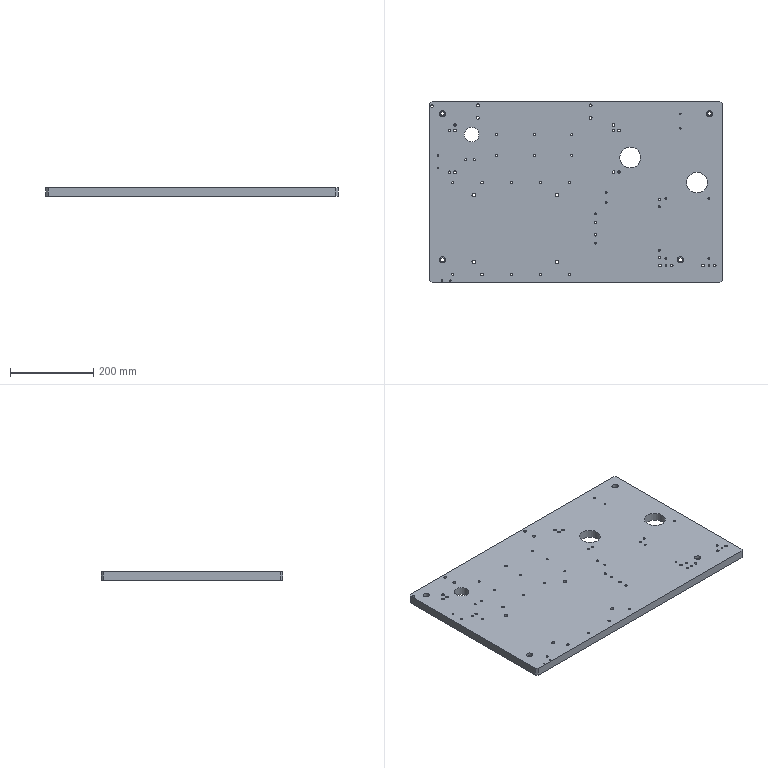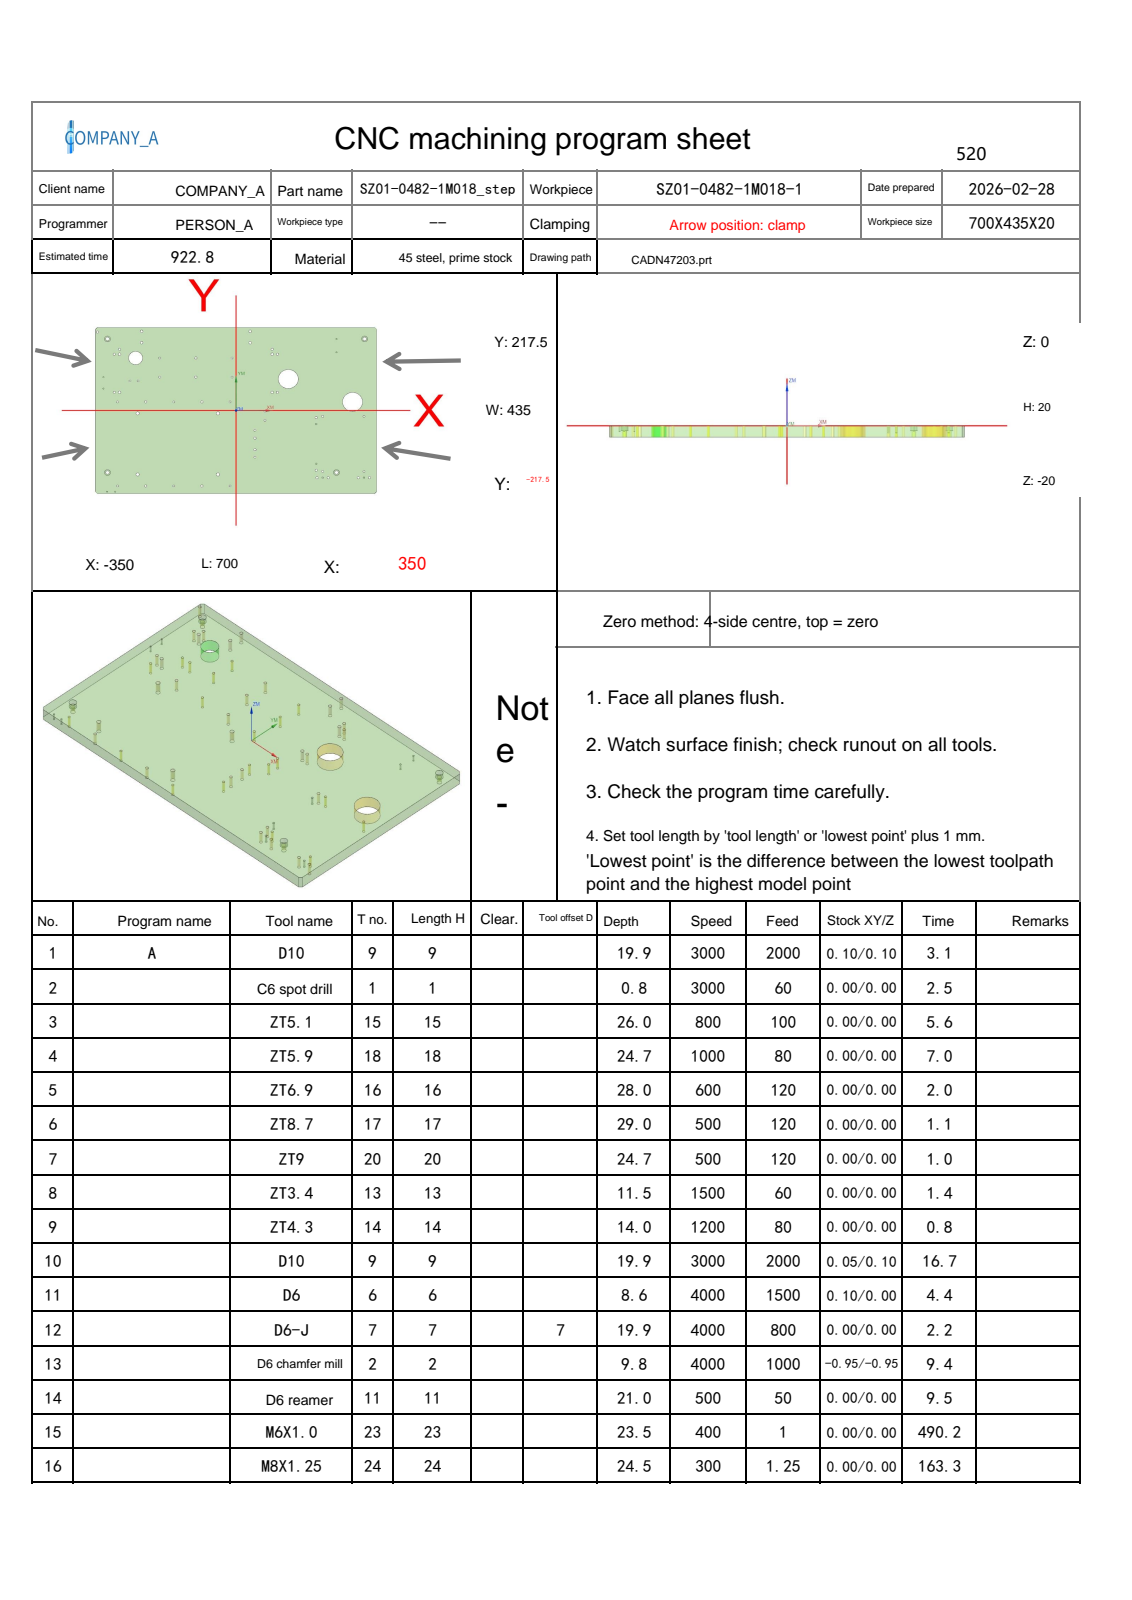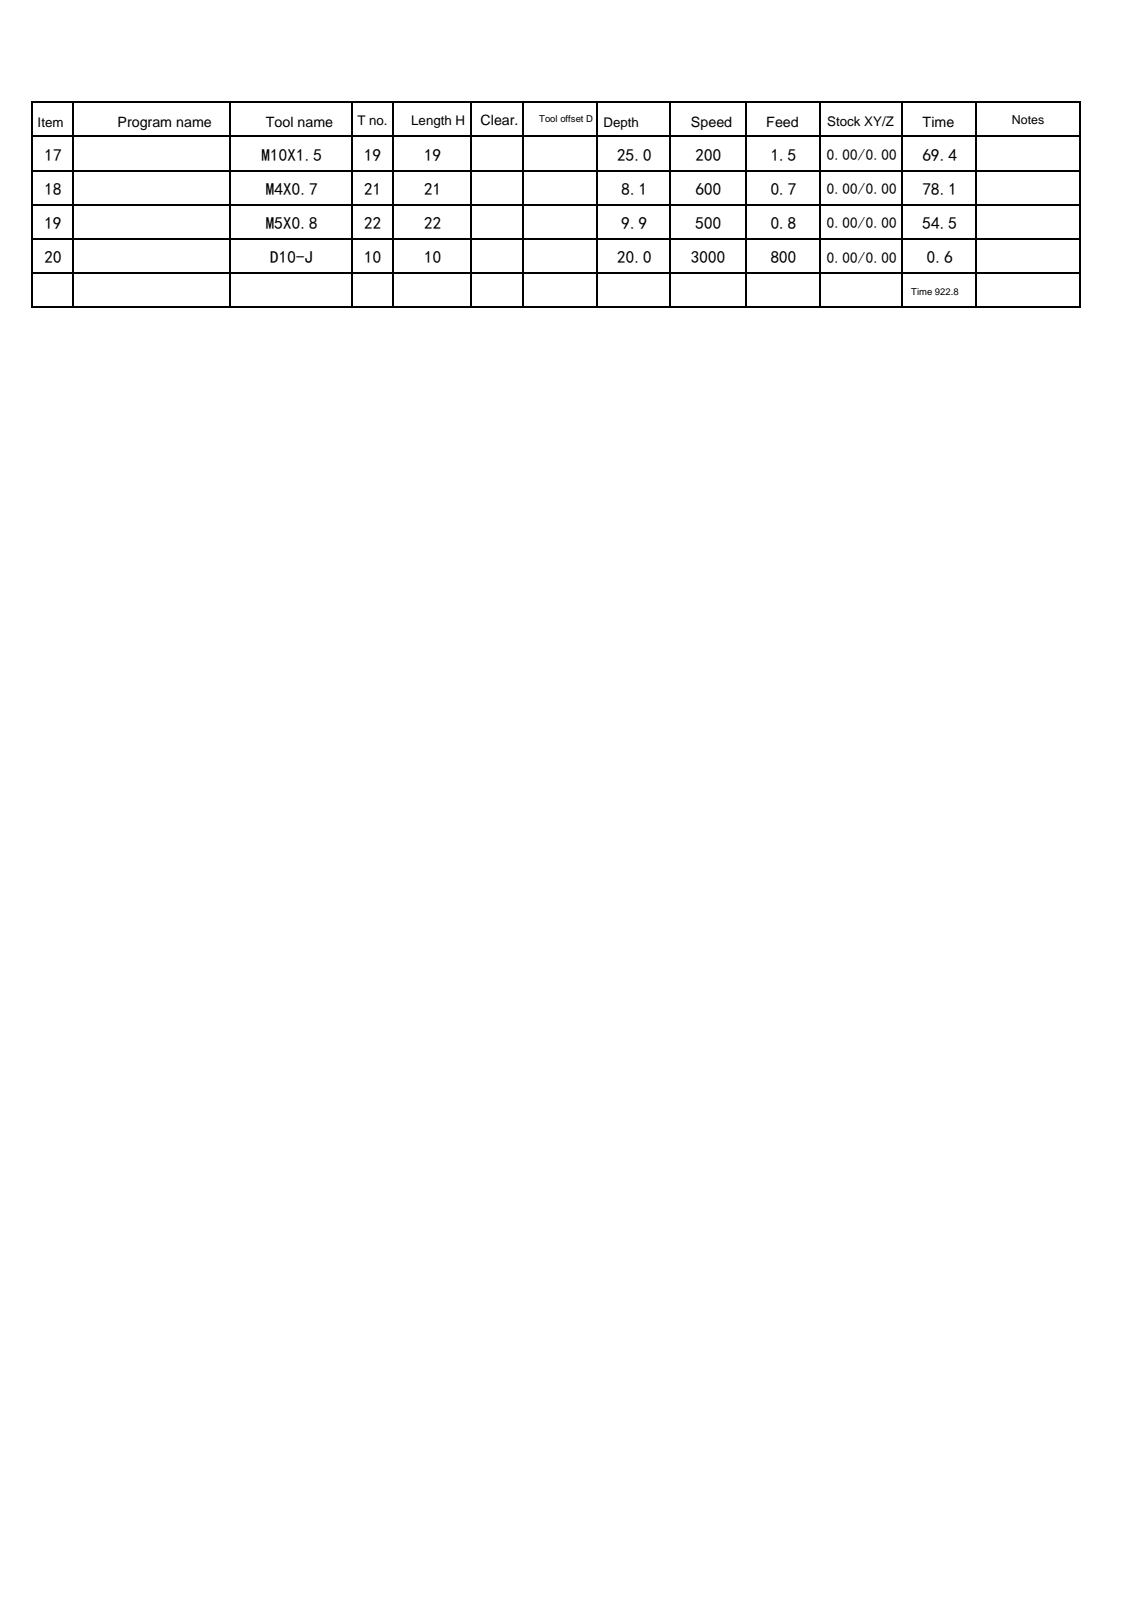NC program | NX | posted by the shop | part box 700 x 435 x 20 mm
Lines 1191 to 2452 of 5271, first 972 of 1262 lines:
N10 T09 M06
(D10  D=10. R=0. H=09 ce=0.05 di=0.10)
G00 G90 G54 X301.511 Y6.205 M03 S3000
G43 H09 Z50.
M08
Z1.
G01 X301.92 Y6.466 Z.975 F2000.
X304.128 Y8.372 Z.822
X306.034 Y10.58 Z.669
X307.599 Y13.041 Z.516
X308.789 Y15.704 Z.363
X309.578 Y18.512 Z.21
X309.95 Y21.406 Z.057
Y22.5 Z0.0
G03 X290. Y42.45 Z-.05 I-19.95 J0.0
X270.05 Y22.5 Z-.099 I0.0 J-19.95
X290. Y2.55 Z-.149 I19.95 J0.0
X309.95 Y22.5 Z-.199 I0.0 J19.95
X290. Y42.45 Z-.248 I-19.95 J0.0
X270.05 Y22.5 Z-.298 I0.0 J-19.95
X290. Y2.55 Z-.347 I19.95 J0.0
X309.95 Y22.5 Z-.397 I0.0 J19.95
X290. Y42.45 Z-.447 I-19.95 J0.0
X270.05 Y22.5 Z-.496 I0.0 J-19.95
X290. Y2.55 Z-.546 I19.95 J0.0
X309.95 Y22.5 Z-.596 I0.0 J19.95
X290. Y42.45 Z-.645 I-19.95 J0.0
X270.05 Y22.5 Z-.695 I0.0 J-19.95
X290. Y2.55 Z-.744 I19.95 J0.0
X309.95 Y22.5 Z-.794 I0.0 J19.95
X290. Y42.45 Z-.844 I-19.95 J0.0
X270.05 Y22.5 Z-.893 I0.0 J-19.95
X290. Y2.55 Z-.943 I19.95 J0.0
X309.95 Y22.5 Z-.993 I0.0 J19.95
X290. Y42.45 Z-1.042 I-19.95 J0.0
X270.05 Y22.5 Z-1.092 I0.0 J-19.95
X290. Y2.55 Z-1.141 I19.95 J0.0
X309.95 Y22.5 Z-1.191 I0.0 J19.95
X290. Y42.45 Z-1.241 I-19.95 J0.0
X270.05 Y22.5 Z-1.29 I0.0 J-19.95
X290. Y2.55 Z-1.34 I19.95 J0.0
X309.95 Y22.5 Z-1.39 I0.0 J19.95
X290. Y42.45 Z-1.439 I-19.95 J0.0
X270.05 Y22.5 Z-1.489 I0.0 J-19.95
X290. Y2.55 Z-1.538 I19.95 J0.0
X309.95 Y22.5 Z-1.588 I0.0 J19.95
X290. Y42.45 Z-1.638 I-19.95 J0.0
X270.05 Y22.5 Z-1.687 I0.0 J-19.95
X290. Y2.55 Z-1.737 I19.95 J0.0
X309.95 Y22.5 Z-1.787 I0.0 J19.95
X290. Y42.45 Z-1.836 I-19.95 J0.0
X270.05 Y22.5 Z-1.886 I0.0 J-19.95
X290. Y2.55 Z-1.935 I19.95 J0.0
X309.95 Y22.5 Z-1.985 I0.0 J19.95
X290. Y42.45 Z-2.035 I-19.95 J0.0
X270.05 Y22.5 Z-2.084 I0.0 J-19.95
X290. Y2.55 Z-2.134 I19.95 J0.0
X309.95 Y22.5 Z-2.184 I0.0 J19.95
X290. Y42.45 Z-2.233 I-19.95 J0.0
X270.05 Y22.5 Z-2.283 I0.0 J-19.95
X290. Y2.55 Z-2.332 I19.95 J0.0
X309.95 Y22.5 Z-2.382 I0.0 J19.95
X290. Y42.45 Z-2.432 I-19.95 J0.0
X270.05 Y22.5 Z-2.481 I0.0 J-19.95
X290. Y2.55 Z-2.531 I19.95 J0.0
X309.95 Y22.5 Z-2.581 I0.0 J19.95
X290. Y42.45 Z-2.63 I-19.95 J0.0
X270.05 Y22.5 Z-2.68 I0.0 J-19.95
X290. Y2.55 Z-2.729 I19.95 J0.0
X309.95 Y22.5 Z-2.779 I0.0 J19.95
X290. Y42.45 Z-2.829 I-19.95 J0.0
X270.05 Y22.5 Z-2.878 I0.0 J-19.95
X290. Y2.55 Z-2.928 I19.95 J0.0
X309.95 Y22.5 Z-2.978 I0.0 J19.95
X290. Y42.45 Z-3.027 I-19.95 J0.0
X270.05 Y22.5 Z-3.077 I0.0 J-19.95
X290. Y2.55 Z-3.126 I19.95 J0.0
X309.95 Y22.5 Z-3.176 I0.0 J19.95
X290. Y42.45 Z-3.226 I-19.95 J0.0
X270.05 Y22.5 Z-3.275 I0.0 J-19.95
X290. Y2.55 Z-3.325 I19.95 J0.0
X309.95 Y22.5 Z-3.375 I0.0 J19.95
X290. Y42.45 Z-3.424 I-19.95 J0.0
X270.05 Y22.5 Z-3.474 I0.0 J-19.95
X290. Y2.55 Z-3.523 I19.95 J0.0
X309.95 Y22.5 Z-3.573 I0.0 J19.95
X290. Y42.45 Z-3.623 I-19.95 J0.0
X270.05 Y22.5 Z-3.672 I0.0 J-19.95
X290. Y2.55 Z-3.722 I19.95 J0.0
X309.95 Y22.5 Z-3.772 I0.0 J19.95
X290. Y42.45 Z-3.821 I-19.95 J0.0
X270.05 Y22.5 Z-3.871 I0.0 J-19.95
X290. Y2.55 Z-3.92 I19.95 J0.0
X309.95 Y22.5 Z-3.97 I0.0 J19.95
X290. Y42.45 Z-4.02 I-19.95 J0.0
X270.05 Y22.5 Z-4.069 I0.0 J-19.95
X290. Y2.55 Z-4.119 I19.95 J0.0
X309.95 Y22.5 Z-4.169 I0.0 J19.95
X290. Y42.45 Z-4.218 I-19.95 J0.0
X270.05 Y22.5 Z-4.268 I0.0 J-19.95
X290. Y2.55 Z-4.317 I19.95 J0.0
X309.95 Y22.5 Z-4.367 I0.0 J19.95
X290. Y42.45 Z-4.417 I-19.95 J0.0
X270.05 Y22.5 Z-4.466 I0.0 J-19.95
X290. Y2.55 Z-4.516 I19.95 J0.0
X309.95 Y22.5 Z-4.566 I0.0 J19.95
X290. Y42.45 Z-4.615 I-19.95 J0.0
X270.05 Y22.5 Z-4.665 I0.0 J-19.95
X290. Y2.55 Z-4.714 I19.95 J0.0
X309.95 Y22.5 Z-4.764 I0.0 J19.95
X290. Y42.45 Z-4.814 I-19.95 J0.0
X270.05 Y22.5 Z-4.863 I0.0 J-19.95
X290. Y2.55 Z-4.913 I19.95 J0.0
X309.95 Y22.5 Z-4.963 I0.0 J19.95
X290. Y42.45 Z-5.012 I-19.95 J0.0
X270.05 Y22.5 Z-5.062 I0.0 J-19.95
X290. Y2.55 Z-5.111 I19.95 J0.0
X309.95 Y22.5 Z-5.161 I0.0 J19.95
X290. Y42.45 Z-5.211 I-19.95 J0.0
X270.05 Y22.5 Z-5.26 I0.0 J-19.95
X290. Y2.55 Z-5.31 I19.95 J0.0
X309.95 Y22.5 Z-5.36 I0.0 J19.95
X290. Y42.45 Z-5.409 I-19.95 J0.0
X270.05 Y22.5 Z-5.459 I0.0 J-19.95
X290. Y2.55 Z-5.508 I19.95 J0.0
X309.95 Y22.5 Z-5.558 I0.0 J19.95
X290. Y42.45 Z-5.608 I-19.95 J0.0
X270.05 Y22.5 Z-5.657 I0.0 J-19.95
X290. Y2.55 Z-5.707 I19.95 J0.0
X309.95 Y22.5 Z-5.757 I0.0 J19.95
X290. Y42.45 Z-5.806 I-19.95 J0.0
X270.05 Y22.5 Z-5.856 I0.0 J-19.95
X290. Y2.55 Z-5.905 I19.95 J0.0
X309.95 Y22.5 Z-5.955 I0.0 J19.95
X290. Y42.45 Z-6.005 I-19.95 J0.0
X270.05 Y22.5 Z-6.054 I0.0 J-19.95
X290. Y2.55 Z-6.104 I19.95 J0.0
X309.95 Y22.5 Z-6.154 I0.0 J19.95
X290. Y42.45 Z-6.203 I-19.95 J0.0
X270.05 Y22.5 Z-6.253 I0.0 J-19.95
X290. Y2.55 Z-6.302 I19.95 J0.0
X309.95 Y22.5 Z-6.352 I0.0 J19.95
X290. Y42.45 Z-6.402 I-19.95 J0.0
X270.05 Y22.5 Z-6.451 I0.0 J-19.95
X290. Y2.55 Z-6.501 I19.95 J0.0
X309.95 Y22.5 Z-6.551 I0.0 J19.95
X290. Y42.45 Z-6.6 I-19.95 J0.0
X270.05 Y22.5 Z-6.65 I0.0 J-19.95
X290. Y2.55 Z-6.699 I19.95 J0.0
X309.95 Y22.5 Z-6.749 I0.0 J19.95
X290. Y42.45 Z-6.799 I-19.95 J0.0
X270.05 Y22.5 Z-6.848 I0.0 J-19.95
X290. Y2.55 Z-6.898 I19.95 J0.0
X309.95 Y22.5 Z-6.948 I0.0 J19.95
X290. Y42.45 Z-6.997 I-19.95 J0.0
X270.05 Y22.5 Z-7.047 I0.0 J-19.95
X290. Y2.55 Z-7.096 I19.95 J0.0
X309.95 Y22.5 Z-7.146 I0.0 J19.95
X290. Y42.45 Z-7.196 I-19.95 J0.0
X270.05 Y22.5 Z-7.245 I0.0 J-19.95
X290. Y2.55 Z-7.295 I19.95 J0.0
X309.95 Y22.5 Z-7.345 I0.0 J19.95
X290. Y42.45 Z-7.394 I-19.95 J0.0
X270.05 Y22.5 Z-7.444 I0.0 J-19.95
X290. Y2.55 Z-7.493 I19.95 J0.0
X309.95 Y22.5 Z-7.543 I0.0 J19.95
X290. Y42.45 Z-7.593 I-19.95 J0.0
X270.05 Y22.5 Z-7.642 I0.0 J-19.95
X290. Y2.55 Z-7.692 I19.95 J0.0
X309.95 Y22.5 Z-7.742 I0.0 J19.95
X290. Y42.45 Z-7.791 I-19.95 J0.0
X270.05 Y22.5 Z-7.841 I0.0 J-19.95
X290. Y2.55 Z-7.89 I19.95 J0.0
X309.95 Y22.5 Z-7.94 I0.0 J19.95
X290. Y42.45 Z-7.99 I-19.95 J0.0
X270.05 Y22.5 Z-8.039 I0.0 J-19.95
X290. Y2.55 Z-8.089 I19.95 J0.0
X309.95 Y22.5 Z-8.139 I0.0 J19.95
X290. Y42.45 Z-8.188 I-19.95 J0.0
X270.05 Y22.5 Z-8.238 I0.0 J-19.95
X290. Y2.55 Z-8.287 I19.95 J0.0
X309.95 Y22.5 Z-8.337 I0.0 J19.95
X290. Y42.45 Z-8.387 I-19.95 J0.0
X270.05 Y22.5 Z-8.436 I0.0 J-19.95
X290. Y2.55 Z-8.486 I19.95 J0.0
X309.95 Y22.5 Z-8.536 I0.0 J19.95
X290. Y42.45 Z-8.585 I-19.95 J0.0
X270.05 Y22.5 Z-8.635 I0.0 J-19.95
X290. Y2.55 Z-8.684 I19.95 J0.0
X309.95 Y22.5 Z-8.734 I0.0 J19.95
X290. Y42.45 Z-8.784 I-19.95 J0.0
X270.05 Y22.5 Z-8.833 I0.0 J-19.95
X290. Y2.55 Z-8.883 I19.95 J0.0
X309.95 Y22.5 Z-8.933 I0.0 J19.95
X290. Y42.45 Z-8.982 I-19.95 J0.0
X270.05 Y22.5 Z-9.032 I0.0 J-19.95
X290. Y2.55 Z-9.081 I19.95 J0.0
X309.95 Y22.5 Z-9.131 I0.0 J19.95
X290. Y42.45 Z-9.181 I-19.95 J0.0
X270.05 Y22.5 Z-9.23 I0.0 J-19.95
X290. Y2.55 Z-9.28 I19.95 J0.0
X309.95 Y22.5 Z-9.33 I0.0 J19.95
X290. Y42.45 Z-9.379 I-19.95 J0.0
X270.05 Y22.5 Z-9.429 I0.0 J-19.95
X290. Y2.55 Z-9.478 I19.95 J0.0
X309.95 Y22.5 Z-9.528 I0.0 J19.95
X290. Y42.45 Z-9.578 I-19.95 J0.0
X270.05 Y22.5 Z-9.627 I0.0 J-19.95
X290. Y2.55 Z-9.677 I19.95 J0.0
X309.95 Y22.5 Z-9.727 I0.0 J19.95
X290. Y42.45 Z-9.776 I-19.95 J0.0
X270.05 Y22.5 Z-9.826 I0.0 J-19.95
X290. Y2.55 Z-9.875 I19.95 J0.0
X309.95 Y22.5 Z-9.925 I0.0 J19.95
X290. Y42.45 Z-9.975 I-19.95 J0.0
X270.05 Y22.5 Z-10.024 I0.0 J-19.95
X290. Y2.55 Z-10.074 I19.95 J0.0
X309.95 Y22.5 Z-10.124 I0.0 J19.95
X290. Y42.45 Z-10.173 I-19.95 J0.0
X270.05 Y22.5 Z-10.223 I0.0 J-19.95
X290. Y2.55 Z-10.272 I19.95 J0.0
X309.95 Y22.5 Z-10.322 I0.0 J19.95
X290. Y42.45 Z-10.372 I-19.95 J0.0
X270.05 Y22.5 Z-10.421 I0.0 J-19.95
X290. Y2.55 Z-10.471 I19.95 J0.0
X309.95 Y22.5 Z-10.521 I0.0 J19.95
X290. Y42.45 Z-10.57 I-19.95 J0.0
X270.05 Y22.5 Z-10.62 I0.0 J-19.95
X290. Y2.55 Z-10.669 I19.95 J0.0
X309.95 Y22.5 Z-10.719 I0.0 J19.95
X290. Y42.45 Z-10.769 I-19.95 J0.0
X270.05 Y22.5 Z-10.818 I0.0 J-19.95
X290. Y2.55 Z-10.868 I19.95 J0.0
X309.95 Y22.5 Z-10.918 I0.0 J19.95
X290. Y42.45 Z-10.967 I-19.95 J0.0
X270.05 Y22.5 Z-11.017 I0.0 J-19.95
X290. Y2.55 Z-11.066 I19.95 J0.0
X309.95 Y22.5 Z-11.116 I0.0 J19.95
X290. Y42.45 Z-11.166 I-19.95 J0.0
X270.05 Y22.5 Z-11.215 I0.0 J-19.95
X290. Y2.55 Z-11.265 I19.95 J0.0
X309.95 Y22.5 Z-11.315 I0.0 J19.95
X290. Y42.45 Z-11.364 I-19.95 J0.0
X270.05 Y22.5 Z-11.414 I0.0 J-19.95
X290. Y2.55 Z-11.463 I19.95 J0.0
X309.95 Y22.5 Z-11.513 I0.0 J19.95
X290. Y42.45 Z-11.563 I-19.95 J0.0
X270.05 Y22.5 Z-11.612 I0.0 J-19.95
X290. Y2.55 Z-11.662 I19.95 J0.0
X309.95 Y22.5 Z-11.712 I0.0 J19.95
X290. Y42.45 Z-11.761 I-19.95 J0.0
X270.05 Y22.5 Z-11.811 I0.0 J-19.95
X290. Y2.55 Z-11.86 I19.95 J0.0
X309.95 Y22.5 Z-11.91 I0.0 J19.95
X290. Y42.45 Z-11.96 I-19.95 J0.0
X270.05 Y22.5 Z-12.009 I0.0 J-19.95
X290. Y2.55 Z-12.059 I19.95 J0.0
X309.95 Y22.5 Z-12.109 I0.0 J19.95
X290. Y42.45 Z-12.158 I-19.95 J0.0
X270.05 Y22.5 Z-12.208 I0.0 J-19.95
X290. Y2.55 Z-12.257 I19.95 J0.0
X309.95 Y22.5 Z-12.307 I0.0 J19.95
X290. Y42.45 Z-12.357 I-19.95 J0.0
X270.05 Y22.5 Z-12.406 I0.0 J-19.95
X290. Y2.55 Z-12.456 I19.95 J0.0
X309.95 Y22.5 Z-12.506 I0.0 J19.95
X290. Y42.45 Z-12.555 I-19.95 J0.0
X270.05 Y22.5 Z-12.605 I0.0 J-19.95
X290. Y2.55 Z-12.654 I19.95 J0.0
X309.95 Y22.5 Z-12.704 I0.0 J19.95
X290. Y42.45 Z-12.754 I-19.95 J0.0
X270.05 Y22.5 Z-12.803 I0.0 J-19.95
X290. Y2.55 Z-12.853 I19.95 J0.0
X309.95 Y22.5 Z-12.903 I0.0 J19.95
X290. Y42.45 Z-12.952 I-19.95 J0.0
X270.05 Y22.5 Z-13.002 I0.0 J-19.95
X290. Y2.55 Z-13.051 I19.95 J0.0
X309.95 Y22.5 Z-13.101 I0.0 J19.95
X290. Y42.45 Z-13.151 I-19.95 J0.0
X270.05 Y22.5 Z-13.2 I0.0 J-19.95
X290. Y2.55 Z-13.25 I19.95 J0.0
X309.95 Y22.5 Z-13.3 I0.0 J19.95
X290. Y42.45 Z-13.349 I-19.95 J0.0
X270.05 Y22.5 Z-13.399 I0.0 J-19.95
X290. Y2.55 Z-13.448 I19.95 J0.0
X309.95 Y22.5 Z-13.498 I0.0 J19.95
X290. Y42.45 Z-13.548 I-19.95 J0.0
X270.05 Y22.5 Z-13.597 I0.0 J-19.95
X290. Y2.55 Z-13.647 I19.95 J0.0
X309.95 Y22.5 Z-13.697 I0.0 J19.95
X290. Y42.45 Z-13.746 I-19.95 J0.0
X270.05 Y22.5 Z-13.796 I0.0 J-19.95
X290. Y2.55 Z-13.845 I19.95 J0.0
X309.95 Y22.5 Z-13.895 I0.0 J19.95
X290. Y42.45 Z-13.945 I-19.95 J0.0
X270.05 Y22.5 Z-13.994 I0.0 J-19.95
X290. Y2.55 Z-14.044 I19.95 J0.0
X309.95 Y22.5 Z-14.094 I0.0 J19.95
X290. Y42.45 Z-14.143 I-19.95 J0.0
X270.05 Y22.5 Z-14.193 I0.0 J-19.95
X290. Y2.55 Z-14.242 I19.95 J0.0
X309.95 Y22.5 Z-14.292 I0.0 J19.95
X290. Y42.45 Z-14.342 I-19.95 J0.0
X270.05 Y22.5 Z-14.391 I0.0 J-19.95
X290. Y2.55 Z-14.441 I19.95 J0.0
X309.95 Y22.5 Z-14.491 I0.0 J19.95
X290. Y42.45 Z-14.54 I-19.95 J0.0
X270.05 Y22.5 Z-14.59 I0.0 J-19.95
X290. Y2.55 Z-14.639 I19.95 J0.0
X309.95 Y22.5 Z-14.689 I0.0 J19.95
X290. Y42.45 Z-14.739 I-19.95 J0.0
X270.05 Y22.5 Z-14.788 I0.0 J-19.95
X290. Y2.55 Z-14.838 I19.95 J0.0
X309.95 Y22.5 Z-14.888 I0.0 J19.95
X290. Y42.45 Z-14.937 I-19.95 J0.0
X270.05 Y22.5 Z-14.987 I0.0 J-19.95
X290. Y2.55 Z-15.036 I19.95 J0.0
X309.95 Y22.5 Z-15.086 I0.0 J19.95
X290. Y42.45 Z-15.136 I-19.95 J0.0
X270.05 Y22.5 Z-15.185 I0.0 J-19.95
X290. Y2.55 Z-15.235 I19.95 J0.0
X309.95 Y22.5 Z-15.285 I0.0 J19.95
X290. Y42.45 Z-15.334 I-19.95 J0.0
X270.05 Y22.5 Z-15.384 I0.0 J-19.95
X290. Y2.55 Z-15.433 I19.95 J0.0
X309.95 Y22.5 Z-15.483 I0.0 J19.95
X290. Y42.45 Z-15.533 I-19.95 J0.0
X270.05 Y22.5 Z-15.582 I0.0 J-19.95
X290. Y2.55 Z-15.632 I19.95 J0.0
X309.95 Y22.5 Z-15.682 I0.0 J19.95
X290. Y42.45 Z-15.731 I-19.95 J0.0
X270.05 Y22.5 Z-15.781 I0.0 J-19.95
X290. Y2.55 Z-15.83 I19.95 J0.0
X309.95 Y22.5 Z-15.88 I0.0 J19.95
X290. Y42.45 Z-15.93 I-19.95 J0.0
X270.05 Y22.5 Z-15.979 I0.0 J-19.95
X290. Y2.55 Z-16.029 I19.95 J0.0
X309.95 Y22.5 Z-16.079 I0.0 J19.95
X290. Y42.45 Z-16.128 I-19.95 J0.0
X270.05 Y22.5 Z-16.178 I0.0 J-19.95
X290. Y2.55 Z-16.227 I19.95 J0.0
X309.95 Y22.5 Z-16.277 I0.0 J19.95
X290. Y42.45 Z-16.327 I-19.95 J0.0
X270.05 Y22.5 Z-16.376 I0.0 J-19.95
X290. Y2.55 Z-16.426 I19.95 J0.0
X309.95 Y22.5 Z-16.476 I0.0 J19.95
X290. Y42.45 Z-16.525 I-19.95 J0.0
X270.05 Y22.5 Z-16.575 I0.0 J-19.95
X290. Y2.55 Z-16.624 I19.95 J0.0
X309.95 Y22.5 Z-16.674 I0.0 J19.95
X290. Y42.45 Z-16.724 I-19.95 J0.0
X270.05 Y22.5 Z-16.773 I0.0 J-19.95
X290. Y2.55 Z-16.823 I19.95 J0.0
X309.95 Y22.5 Z-16.873 I0.0 J19.95
X290. Y42.45 Z-16.922 I-19.95 J0.0
X270.05 Y22.5 Z-16.972 I0.0 J-19.95
X290. Y2.55 Z-17.021 I19.95 J0.0
X309.95 Y22.5 Z-17.071 I0.0 J19.95
X290. Y42.45 Z-17.121 I-19.95 J0.0
X270.05 Y22.5 Z-17.17 I0.0 J-19.95
X290. Y2.55 Z-17.22 I19.95 J0.0
X309.95 Y22.5 Z-17.27 I0.0 J19.95
X290. Y42.45 Z-17.319 I-19.95 J0.0
X270.05 Y22.5 Z-17.369 I0.0 J-19.95
X290. Y2.55 Z-17.418 I19.95 J0.0
X309.95 Y22.5 Z-17.468 I0.0 J19.95
X290. Y42.45 Z-17.518 I-19.95 J0.0
X270.05 Y22.5 Z-17.567 I0.0 J-19.95
X290. Y2.55 Z-17.617 I19.95 J0.0
X309.95 Y22.5 Z-17.667 I0.0 J19.95
X290. Y42.45 Z-17.716 I-19.95 J0.0
X270.05 Y22.5 Z-17.766 I0.0 J-19.95
X290. Y2.55 Z-17.815 I19.95 J0.0
X309.95 Y22.5 Z-17.865 I0.0 J19.95
X290. Y42.45 Z-17.915 I-19.95 J0.0
X270.05 Y22.5 Z-17.964 I0.0 J-19.95
X290. Y2.55 Z-18.014 I19.95 J0.0
X309.95 Y22.5 Z-18.064 I0.0 J19.95
X290. Y42.45 Z-18.113 I-19.95 J0.0
X270.05 Y22.5 Z-18.163 I0.0 J-19.95
X290. Y2.55 Z-18.212 I19.95 J0.0
X309.95 Y22.5 Z-18.262 I0.0 J19.95
X290. Y42.45 Z-18.312 I-19.95 J0.0
X270.05 Y22.5 Z-18.361 I0.0 J-19.95
X290. Y2.55 Z-18.411 I19.95 J0.0
X309.95 Y22.5 Z-18.461 I0.0 J19.95
X290. Y42.45 Z-18.51 I-19.95 J0.0
X270.05 Y22.5 Z-18.56 I0.0 J-19.95
X290. Y2.55 Z-18.609 I19.95 J0.0
X309.95 Y22.5 Z-18.659 I0.0 J19.95
X290. Y42.45 Z-18.709 I-19.95 J0.0
X270.05 Y22.5 Z-18.758 I0.0 J-19.95
X290. Y2.55 Z-18.808 I19.95 J0.0
X309.95 Y22.5 Z-18.858 I0.0 J19.95
X290. Y42.45 Z-18.907 I-19.95 J0.0
X270.05 Y22.5 Z-18.957 I0.0 J-19.95
X290. Y2.55 Z-19.006 I19.95 J0.0
X309.95 Y22.5 Z-19.056 I0.0 J19.95
X290. Y42.45 Z-19.106 I-19.95 J0.0
X270.05 Y22.5 Z-19.155 I0.0 J-19.95
X290. Y2.55 Z-19.205 I19.95 J0.0
X309.95 Y22.5 Z-19.255 I0.0 J19.95
X290. Y42.45 Z-19.304 I-19.95 J0.0
X270.05 Y22.5 Z-19.354 I0.0 J-19.95
X290. Y2.55 Z-19.403 I19.95 J0.0
X309.95 Y22.5 Z-19.453 I0.0 J19.95
X290. Y42.45 Z-19.503 I-19.95 J0.0
X270.05 Y22.5 Z-19.552 I0.0 J-19.95
X290. Y2.55 Z-19.602 I19.95 J0.0
X309.95 Y22.5 Z-19.652 I0.0 J19.95
X290. Y42.45 Z-19.701 I-19.95 J0.0
X270.05 Y22.5 Z-19.751 I0.0 J-19.95
X290. Y2.55 Z-19.8 I19.95 J0.0
X309.95 Y22.5 Z-19.85 I0.0 J19.95
X290. Y42.45 I-19.95 J0.0
X270.05 Y22.5 I0.0 J-19.95
X290. Y2.55 I19.95 J0.0
X309.95 Y22.5 I0.0 J19.95
X309.946 Y22.9 I-19.95 J0.0
G01 Z-18.85
G00 Z50.
X146.295 Y94.011
Z1.
G01 X146.034 Y94.42 Z.975
X144.128 Y96.628 Z.822
X141.92 Y98.534 Z.669
X139.459 Y100.099 Z.516
X136.796 Y101.289 Z.363
X133.988 Y102.078 Z.21
X131.094 Y102.45 Z.057
X130. Z0.0
G03 X110.05 Y82.5 Z-.05 I0.0 J-19.95
X130. Y62.55 Z-.099 I19.95 J0.0
X149.95 Y82.5 Z-.149 I0.0 J19.95
X130. Y102.45 Z-.199 I-19.95 J0.0
X110.05 Y82.5 Z-.248 I0.0 J-19.95
X130. Y62.55 Z-.298 I19.95 J0.0
X149.95 Y82.5 Z-.347 I0.0 J19.95
X130. Y102.45 Z-.397 I-19.95 J0.0
X110.05 Y82.5 Z-.447 I0.0 J-19.95
X130. Y62.55 Z-.496 I19.95 J0.0
X149.95 Y82.5 Z-.546 I0.0 J19.95
X130. Y102.45 Z-.596 I-19.95 J0.0
X110.05 Y82.5 Z-.645 I0.0 J-19.95
X130. Y62.55 Z-.695 I19.95 J0.0
X149.95 Y82.5 Z-.744 I0.0 J19.95
X130. Y102.45 Z-.794 I-19.95 J0.0
X110.05 Y82.5 Z-.844 I0.0 J-19.95
X130. Y62.55 Z-.893 I19.95 J0.0
X149.95 Y82.5 Z-.943 I0.0 J19.95
X130. Y102.45 Z-.993 I-19.95 J0.0
X110.05 Y82.5 Z-1.042 I0.0 J-19.95
X130. Y62.55 Z-1.092 I19.95 J0.0
X149.95 Y82.5 Z-1.141 I0.0 J19.95
X130. Y102.45 Z-1.191 I-19.95 J0.0
X110.05 Y82.5 Z-1.241 I0.0 J-19.95
X130. Y62.55 Z-1.29 I19.95 J0.0
X149.95 Y82.5 Z-1.34 I0.0 J19.95
X130. Y102.45 Z-1.39 I-19.95 J0.0
X110.05 Y82.5 Z-1.439 I0.0 J-19.95
X130. Y62.55 Z-1.489 I19.95 J0.0
X149.95 Y82.5 Z-1.538 I0.0 J19.95
X130. Y102.45 Z-1.588 I-19.95 J0.0
X110.05 Y82.5 Z-1.638 I0.0 J-19.95
X130. Y62.55 Z-1.687 I19.95 J0.0
X149.95 Y82.5 Z-1.737 I0.0 J19.95
X130. Y102.45 Z-1.787 I-19.95 J0.0
X110.05 Y82.5 Z-1.836 I0.0 J-19.95
X130. Y62.55 Z-1.886 I19.95 J0.0
X149.95 Y82.5 Z-1.935 I0.0 J19.95
X130. Y102.45 Z-1.985 I-19.95 J0.0
X110.05 Y82.5 Z-2.035 I0.0 J-19.95
X130. Y62.55 Z-2.084 I19.95 J0.0
X149.95 Y82.5 Z-2.134 I0.0 J19.95
X130. Y102.45 Z-2.184 I-19.95 J0.0
X110.05 Y82.5 Z-2.233 I0.0 J-19.95
X130. Y62.55 Z-2.283 I19.95 J0.0
X149.95 Y82.5 Z-2.332 I0.0 J19.95
X130. Y102.45 Z-2.382 I-19.95 J0.0
X110.05 Y82.5 Z-2.432 I0.0 J-19.95
X130. Y62.55 Z-2.481 I19.95 J0.0
X149.95 Y82.5 Z-2.531 I0.0 J19.95
X130. Y102.45 Z-2.581 I-19.95 J0.0
X110.05 Y82.5 Z-2.63 I0.0 J-19.95
X130. Y62.55 Z-2.68 I19.95 J0.0
X149.95 Y82.5 Z-2.729 I0.0 J19.95
X130. Y102.45 Z-2.779 I-19.95 J0.0
X110.05 Y82.5 Z-2.829 I0.0 J-19.95
X130. Y62.55 Z-2.878 I19.95 J0.0
X149.95 Y82.5 Z-2.928 I0.0 J19.95
X130. Y102.45 Z-2.978 I-19.95 J0.0
X110.05 Y82.5 Z-3.027 I0.0 J-19.95
X130. Y62.55 Z-3.077 I19.95 J0.0
X149.95 Y82.5 Z-3.126 I0.0 J19.95
X130. Y102.45 Z-3.176 I-19.95 J0.0
X110.05 Y82.5 Z-3.226 I0.0 J-19.95
X130. Y62.55 Z-3.275 I19.95 J0.0
X149.95 Y82.5 Z-3.325 I0.0 J19.95
X130. Y102.45 Z-3.375 I-19.95 J0.0
X110.05 Y82.5 Z-3.424 I0.0 J-19.95
X130. Y62.55 Z-3.474 I19.95 J0.0
X149.95 Y82.5 Z-3.523 I0.0 J19.95
X130. Y102.45 Z-3.573 I-19.95 J0.0
X110.05 Y82.5 Z-3.623 I0.0 J-19.95
X130. Y62.55 Z-3.672 I19.95 J0.0
X149.95 Y82.5 Z-3.722 I0.0 J19.95
X130. Y102.45 Z-3.772 I-19.95 J0.0
X110.05 Y82.5 Z-3.821 I0.0 J-19.95
X130. Y62.55 Z-3.871 I19.95 J0.0
X149.95 Y82.5 Z-3.92 I0.0 J19.95
X130. Y102.45 Z-3.97 I-19.95 J0.0
X110.05 Y82.5 Z-4.02 I0.0 J-19.95
X130. Y62.55 Z-4.069 I19.95 J0.0
X149.95 Y82.5 Z-4.119 I0.0 J19.95
X130. Y102.45 Z-4.169 I-19.95 J0.0
X110.05 Y82.5 Z-4.218 I0.0 J-19.95
X130. Y62.55 Z-4.268 I19.95 J0.0
X149.95 Y82.5 Z-4.317 I0.0 J19.95
X130. Y102.45 Z-4.367 I-19.95 J0.0
X110.05 Y82.5 Z-4.417 I0.0 J-19.95
X130. Y62.55 Z-4.466 I19.95 J0.0
X149.95 Y82.5 Z-4.516 I0.0 J19.95
X130. Y102.45 Z-4.566 I-19.95 J0.0
X110.05 Y82.5 Z-4.615 I0.0 J-19.95
X130. Y62.55 Z-4.665 I19.95 J0.0
X149.95 Y82.5 Z-4.714 I0.0 J19.95
X130. Y102.45 Z-4.764 I-19.95 J0.0
X110.05 Y82.5 Z-4.814 I0.0 J-19.95
X130. Y62.55 Z-4.863 I19.95 J0.0
X149.95 Y82.5 Z-4.913 I0.0 J19.95
X130. Y102.45 Z-4.963 I-19.95 J0.0
X110.05 Y82.5 Z-5.012 I0.0 J-19.95
X130. Y62.55 Z-5.062 I19.95 J0.0
X149.95 Y82.5 Z-5.111 I0.0 J19.95
X130. Y102.45 Z-5.161 I-19.95 J0.0
X110.05 Y82.5 Z-5.211 I0.0 J-19.95
X130. Y62.55 Z-5.26 I19.95 J0.0
X149.95 Y82.5 Z-5.31 I0.0 J19.95
X130. Y102.45 Z-5.36 I-19.95 J0.0
X110.05 Y82.5 Z-5.409 I0.0 J-19.95
X130. Y62.55 Z-5.459 I19.95 J0.0
X149.95 Y82.5 Z-5.508 I0.0 J19.95
X130. Y102.45 Z-5.558 I-19.95 J0.0
X110.05 Y82.5 Z-5.608 I0.0 J-19.95
X130. Y62.55 Z-5.657 I19.95 J0.0
X149.95 Y82.5 Z-5.707 I0.0 J19.95
X130. Y102.45 Z-5.757 I-19.95 J0.0
X110.05 Y82.5 Z-5.806 I0.0 J-19.95
X130. Y62.55 Z-5.856 I19.95 J0.0
X149.95 Y82.5 Z-5.905 I0.0 J19.95
X130. Y102.45 Z-5.955 I-19.95 J0.0
X110.05 Y82.5 Z-6.005 I0.0 J-19.95
X130. Y62.55 Z-6.054 I19.95 J0.0
X149.95 Y82.5 Z-6.104 I0.0 J19.95
X130. Y102.45 Z-6.154 I-19.95 J0.0
X110.05 Y82.5 Z-6.203 I0.0 J-19.95
X130. Y62.55 Z-6.253 I19.95 J0.0
X149.95 Y82.5 Z-6.302 I0.0 J19.95
X130. Y102.45 Z-6.352 I-19.95 J0.0
X110.05 Y82.5 Z-6.402 I0.0 J-19.95
X130. Y62.55 Z-6.451 I19.95 J0.0
X149.95 Y82.5 Z-6.501 I0.0 J19.95
X130. Y102.45 Z-6.551 I-19.95 J0.0
X110.05 Y82.5 Z-6.6 I0.0 J-19.95
X130. Y62.55 Z-6.65 I19.95 J0.0
X149.95 Y82.5 Z-6.699 I0.0 J19.95
X130. Y102.45 Z-6.749 I-19.95 J0.0
X110.05 Y82.5 Z-6.799 I0.0 J-19.95
X130. Y62.55 Z-6.848 I19.95 J0.0
X149.95 Y82.5 Z-6.898 I0.0 J19.95
X130. Y102.45 Z-6.948 I-19.95 J0.0
X110.05 Y82.5 Z-6.997 I0.0 J-19.95
X130. Y62.55 Z-7.047 I19.95 J0.0
X149.95 Y82.5 Z-7.096 I0.0 J19.95
X130. Y102.45 Z-7.146 I-19.95 J0.0
X110.05 Y82.5 Z-7.196 I0.0 J-19.95
X130. Y62.55 Z-7.245 I19.95 J0.0
X149.95 Y82.5 Z-7.295 I0.0 J19.95
X130. Y102.45 Z-7.345 I-19.95 J0.0
X110.05 Y82.5 Z-7.394 I0.0 J-19.95
X130. Y62.55 Z-7.444 I19.95 J0.0
X149.95 Y82.5 Z-7.493 I0.0 J19.95
X130. Y102.45 Z-7.543 I-19.95 J0.0
X110.05 Y82.5 Z-7.593 I0.0 J-19.95
X130. Y62.55 Z-7.642 I19.95 J0.0
X149.95 Y82.5 Z-7.692 I0.0 J19.95
X130. Y102.45 Z-7.742 I-19.95 J0.0
X110.05 Y82.5 Z-7.791 I0.0 J-19.95
X130. Y62.55 Z-7.841 I19.95 J0.0
X149.95 Y82.5 Z-7.89 I0.0 J19.95
X130. Y102.45 Z-7.94 I-19.95 J0.0
X110.05 Y82.5 Z-7.99 I0.0 J-19.95
X130. Y62.55 Z-8.039 I19.95 J0.0
X149.95 Y82.5 Z-8.089 I0.0 J19.95
X130. Y102.45 Z-8.139 I-19.95 J0.0
X110.05 Y82.5 Z-8.188 I0.0 J-19.95
X130. Y62.55 Z-8.238 I19.95 J0.0
X149.95 Y82.5 Z-8.287 I0.0 J19.95
X130. Y102.45 Z-8.337 I-19.95 J0.0
X110.05 Y82.5 Z-8.387 I0.0 J-19.95
X130. Y62.55 Z-8.436 I19.95 J0.0
X149.95 Y82.5 Z-8.486 I0.0 J19.95
X130. Y102.45 Z-8.536 I-19.95 J0.0
X110.05 Y82.5 Z-8.585 I0.0 J-19.95
X130. Y62.55 Z-8.635 I19.95 J0.0
X149.95 Y82.5 Z-8.684 I0.0 J19.95
X130. Y102.45 Z-8.734 I-19.95 J0.0
X110.05 Y82.5 Z-8.784 I0.0 J-19.95
X130. Y62.55 Z-8.833 I19.95 J0.0
X149.95 Y82.5 Z-8.883 I0.0 J19.95
X130. Y102.45 Z-8.933 I-19.95 J0.0
X110.05 Y82.5 Z-8.982 I0.0 J-19.95
X130. Y62.55 Z-9.032 I19.95 J0.0
X149.95 Y82.5 Z-9.081 I0.0 J19.95
X130. Y102.45 Z-9.131 I-19.95 J0.0
X110.05 Y82.5 Z-9.181 I0.0 J-19.95
X130. Y62.55 Z-9.23 I19.95 J0.0
X149.95 Y82.5 Z-9.28 I0.0 J19.95
X130. Y102.45 Z-9.33 I-19.95 J0.0
X110.05 Y82.5 Z-9.379 I0.0 J-19.95
X130. Y62.55 Z-9.429 I19.95 J0.0
X149.95 Y82.5 Z-9.478 I0.0 J19.95
X130. Y102.45 Z-9.528 I-19.95 J0.0
X110.05 Y82.5 Z-9.578 I0.0 J-19.95
X130. Y62.55 Z-9.627 I19.95 J0.0
X149.95 Y82.5 Z-9.677 I0.0 J19.95
X130. Y102.45 Z-9.727 I-19.95 J0.0
X110.05 Y82.5 Z-9.776 I0.0 J-19.95
X130. Y62.55 Z-9.826 I19.95 J0.0
X149.95 Y82.5 Z-9.875 I0.0 J19.95
X130. Y102.45 Z-9.925 I-19.95 J0.0
X110.05 Y82.5 Z-9.975 I0.0 J-19.95
X130. Y62.55 Z-10.024 I19.95 J0.0
X149.95 Y82.5 Z-10.074 I0.0 J19.95
X130. Y102.45 Z-10.124 I-19.95 J0.0
X110.05 Y82.5 Z-10.173 I0.0 J-19.95
X130. Y62.55 Z-10.223 I19.95 J0.0
X149.95 Y82.5 Z-10.272 I0.0 J19.95
X130. Y102.45 Z-10.322 I-19.95 J0.0
X110.05 Y82.5 Z-10.372 I0.0 J-19.95
X130. Y62.55 Z-10.421 I19.95 J0.0
X149.95 Y82.5 Z-10.471 I0.0 J19.95
X130. Y102.45 Z-10.521 I-19.95 J0.0
X110.05 Y82.5 Z-10.57 I0.0 J-19.95
X130. Y62.55 Z-10.62 I19.95 J0.0
X149.95 Y82.5 Z-10.669 I0.0 J19.95
X130. Y102.45 Z-10.719 I-19.95 J0.0
X110.05 Y82.5 Z-10.769 I0.0 J-19.95
X130. Y62.55 Z-10.818 I19.95 J0.0
X149.95 Y82.5 Z-10.868 I0.0 J19.95
X130. Y102.45 Z-10.918 I-19.95 J0.0
X110.05 Y82.5 Z-10.967 I0.0 J-19.95
X130. Y62.55 Z-11.017 I19.95 J0.0
X149.95 Y82.5 Z-11.066 I0.0 J19.95
X130. Y102.45 Z-11.116 I-19.95 J0.0
X110.05 Y82.5 Z-11.166 I0.0 J-19.95
X130. Y62.55 Z-11.215 I19.95 J0.0
X149.95 Y82.5 Z-11.265 I0.0 J19.95
X130. Y102.45 Z-11.315 I-19.95 J0.0
X110.05 Y82.5 Z-11.364 I0.0 J-19.95
X130. Y62.55 Z-11.414 I19.95 J0.0
X149.95 Y82.5 Z-11.463 I0.0 J19.95
X130. Y102.45 Z-11.513 I-19.95 J0.0
X110.05 Y82.5 Z-11.563 I0.0 J-19.95
X130. Y62.55 Z-11.612 I19.95 J0.0
X149.95 Y82.5 Z-11.662 I0.0 J19.95
X130. Y102.45 Z-11.712 I-19.95 J0.0
X110.05 Y82.5 Z-11.761 I0.0 J-19.95
X130. Y62.55 Z-11.811 I19.95 J0.0
X149.95 Y82.5 Z-11.86 I0.0 J19.95
X130. Y102.45 Z-11.91 I-19.95 J0.0
X110.05 Y82.5 Z-11.96 I0.0 J-19.95
X130. Y62.55 Z-12.009 I19.95 J0.0
X149.95 Y82.5 Z-12.059 I0.0 J19.95
X130. Y102.45 Z-12.109 I-19.95 J0.0
X110.05 Y82.5 Z-12.158 I0.0 J-19.95
X130. Y62.55 Z-12.208 I19.95 J0.0
X149.95 Y82.5 Z-12.257 I0.0 J19.95
X130. Y102.45 Z-12.307 I-19.95 J0.0
X110.05 Y82.5 Z-12.357 I0.0 J-19.95
X130. Y62.55 Z-12.406 I19.95 J0.0
X149.95 Y82.5 Z-12.456 I0.0 J19.95
X130. Y102.45 Z-12.506 I-19.95 J0.0
X110.05 Y82.5 Z-12.555 I0.0 J-19.95
X130. Y62.55 Z-12.605 I19.95 J0.0
X149.95 Y82.5 Z-12.654 I0.0 J19.95
X130. Y102.45 Z-12.704 I-19.95 J0.0
X110.05 Y82.5 Z-12.754 I0.0 J-19.95
X130. Y62.55 Z-12.803 I19.95 J0.0
X149.95 Y82.5 Z-12.853 I0.0 J19.95
X130. Y102.45 Z-12.903 I-19.95 J0.0
X110.05 Y82.5 Z-12.952 I0.0 J-19.95
X130. Y62.55 Z-13.002 I19.95 J0.0
X149.95 Y82.5 Z-13.051 I0.0 J19.95
X130. Y102.45 Z-13.101 I-19.95 J0.0
X110.05 Y82.5 Z-13.151 I0.0 J-19.95
X130. Y62.55 Z-13.2 I19.95 J0.0
X149.95 Y82.5 Z-13.25 I0.0 J19.95
X130. Y102.45 Z-13.3 I-19.95 J0.0
X110.05 Y82.5 Z-13.349 I0.0 J-19.95
X130. Y62.55 Z-13.399 I19.95 J0.0
X149.95 Y82.5 Z-13.448 I0.0 J19.95
X130. Y102.45 Z-13.498 I-19.95 J0.0
X110.05 Y82.5 Z-13.548 I0.0 J-19.95
X130. Y62.55 Z-13.597 I19.95 J0.0
X149.95 Y82.5 Z-13.647 I0.0 J19.95
X130. Y102.45 Z-13.697 I-19.95 J0.0
X110.05 Y82.5 Z-13.746 I0.0 J-19.95
X130. Y62.55 Z-13.796 I19.95 J0.0
X149.95 Y82.5 Z-13.845 I0.0 J19.95
X130. Y102.45 Z-13.895 I-19.95 J0.0
X110.05 Y82.5 Z-13.945 I0.0 J-19.95
X130. Y62.55 Z-13.994 I19.95 J0.0
X149.95 Y82.5 Z-14.044 I0.0 J19.95
X130. Y102.45 Z-14.094 I-19.95 J0.0
X110.05 Y82.5 Z-14.143 I0.0 J-19.95
X130. Y62.55 Z-14.193 I19.95 J0.0
X149.95 Y82.5 Z-14.242 I0.0 J19.95
X130. Y102.45 Z-14.292 I-19.95 J0.0
X110.05 Y82.5 Z-14.342 I0.0 J-19.95
X130. Y62.55 Z-14.391 I19.95 J0.0
X149.95 Y82.5 Z-14.441 I0.0 J19.95
X130. Y102.45 Z-14.491 I-19.95 J0.0
X110.05 Y82.5 Z-14.54 I0.0 J-19.95
X130. Y62.55 Z-14.59 I19.95 J0.0
X149.95 Y82.5 Z-14.639 I0.0 J19.95
X130. Y102.45 Z-14.689 I-19.95 J0.0
X110.05 Y82.5 Z-14.739 I0.0 J-19.95
X130. Y62.55 Z-14.788 I19.95 J0.0
X149.95 Y82.5 Z-14.838 I0.0 J19.95
X130. Y102.45 Z-14.888 I-19.95 J0.0
X110.05 Y82.5 Z-14.937 I0.0 J-19.95
X130. Y62.55 Z-14.987 I19.95 J0.0
X149.95 Y82.5 Z-15.036 I0.0 J19.95
X130. Y102.45 Z-15.086 I-19.95 J0.0
X110.05 Y82.5 Z-15.136 I0.0 J-19.95
X130. Y62.55 Z-15.185 I19.95 J0.0
X149.95 Y82.5 Z-15.235 I0.0 J19.95
X130. Y102.45 Z-15.285 I-19.95 J0.0
X110.05 Y82.5 Z-15.334 I0.0 J-19.95
X130. Y62.55 Z-15.384 I19.95 J0.0
X149.95 Y82.5 Z-15.433 I0.0 J19.95
X130. Y102.45 Z-15.483 I-19.95 J0.0
X110.05 Y82.5 Z-15.533 I0.0 J-19.95
X130. Y62.55 Z-15.582 I19.95 J0.0
X149.95 Y82.5 Z-15.632 I0.0 J19.95
X130. Y102.45 Z-15.682 I-19.95 J0.0
X110.05 Y82.5 Z-15.731 I0.0 J-19.95
X130. Y62.55 Z-15.781 I19.95 J0.0
X149.95 Y82.5 Z-15.83 I0.0 J19.95
X130. Y102.45 Z-15.88 I-19.95 J0.0
X110.05 Y82.5 Z-15.93 I0.0 J-19.95
X130. Y62.55 Z-15.979 I19.95 J0.0
X149.95 Y82.5 Z-16.029 I0.0 J19.95
X130. Y102.45 Z-16.079 I-19.95 J0.0
X110.05 Y82.5 Z-16.128 I0.0 J-19.95
X130. Y62.55 Z-16.178 I19.95 J0.0
X149.95 Y82.5 Z-16.227 I0.0 J19.95
X130. Y102.45 Z-16.277 I-19.95 J0.0
X110.05 Y82.5 Z-16.327 I0.0 J-19.95
X130. Y62.55 Z-16.376 I19.95 J0.0
X149.95 Y82.5 Z-16.426 I0.0 J19.95
X130. Y102.45 Z-16.476 I-19.95 J0.0
X110.05 Y82.5 Z-16.525 I0.0 J-19.95
X130. Y62.55 Z-16.575 I19.95 J0.0
X149.95 Y82.5 Z-16.624 I0.0 J19.95
X130. Y102.45 Z-16.674 I-19.95 J0.0
X110.05 Y82.5 Z-16.724 I0.0 J-19.95
X130. Y62.55 Z-16.773 I19.95 J0.0
X149.95 Y82.5 Z-16.823 I0.0 J19.95
X130. Y102.45 Z-16.873 I-19.95 J0.0
X110.05 Y82.5 Z-16.922 I0.0 J-19.95
X130. Y62.55 Z-16.972 I19.95 J0.0
X149.95 Y82.5 Z-17.021 I0.0 J19.95
X130. Y102.45 Z-17.071 I-19.95 J0.0
X110.05 Y82.5 Z-17.121 I0.0 J-19.95
X130. Y62.55 Z-17.17 I19.95 J0.0
X149.95 Y82.5 Z-17.22 I0.0 J19.95
X130. Y102.45 Z-17.27 I-19.95 J0.0
X110.05 Y82.5 Z-17.319 I0.0 J-19.95
X130. Y62.55 Z-17.369 I19.95 J0.0
X149.95 Y82.5 Z-17.418 I0.0 J19.95
X130. Y102.45 Z-17.468 I-19.95 J0.0
X110.05 Y82.5 Z-17.518 I0.0 J-19.95
X130. Y62.55 Z-17.567 I19.95 J0.0
X149.95 Y82.5 Z-17.617 I0.0 J19.95
X130. Y102.45 Z-17.667 I-19.95 J0.0
X110.05 Y82.5 Z-17.716 I0.0 J-19.95
X130. Y62.55 Z-17.766 I19.95 J0.0
X149.95 Y82.5 Z-17.815 I0.0 J19.95
X130. Y102.45 Z-17.865 I-19.95 J0.0
X110.05 Y82.5 Z-17.915 I0.0 J-19.95
X130. Y62.55 Z-17.964 I19.95 J0.0
X149.95 Y82.5 Z-18.014 I0.0 J19.95
X130. Y102.45 Z-18.064 I-19.95 J0.0
X110.05 Y82.5 Z-18.113 I0.0 J-19.95
X130. Y62.55 Z-18.163 I19.95 J0.0
X149.95 Y82.5 Z-18.212 I0.0 J19.95
X130. Y102.45 Z-18.262 I-19.95 J0.0
X110.05 Y82.5 Z-18.312 I0.0 J-19.95
X130. Y62.55 Z-18.361 I19.95 J0.0
X149.95 Y82.5 Z-18.411 I0.0 J19.95
X130. Y102.45 Z-18.461 I-19.95 J0.0
X110.05 Y82.5 Z-18.51 I0.0 J-19.95
X130. Y62.55 Z-18.56 I19.95 J0.0
X149.95 Y82.5 Z-18.609 I0.0 J19.95
X130. Y102.45 Z-18.659 I-19.95 J0.0
X110.05 Y82.5 Z-18.709 I0.0 J-19.95
X130. Y62.55 Z-18.758 I19.95 J0.0
X149.95 Y82.5 Z-18.808 I0.0 J19.95
X130. Y102.45 Z-18.858 I-19.95 J0.0
X110.05 Y82.5 Z-18.907 I0.0 J-19.95
X130. Y62.55 Z-18.957 I19.95 J0.0
X149.95 Y82.5 Z-19.006 I0.0 J19.95
X130. Y102.45 Z-19.056 I-19.95 J0.0
X110.05 Y82.5 Z-19.106 I0.0 J-19.95
X130. Y62.55 Z-19.155 I19.95 J0.0
X149.95 Y82.5 Z-19.205 I0.0 J19.95
X130. Y102.45 Z-19.255 I-19.95 J0.0
X110.05 Y82.5 Z-19.304 I0.0 J-19.95
X130. Y62.55 Z-19.354 I19.95 J0.0
X149.95 Y82.5 Z-19.403 I0.0 J19.95
X130. Y102.45 Z-19.453 I-19.95 J0.0
X110.05 Y82.5 Z-19.503 I0.0 J-19.95
X130. Y62.55 Z-19.552 I19.95 J0.0
X149.95 Y82.5 Z-19.602 I0.0 J19.95
X130. Y102.45 Z-19.652 I-19.95 J0.0
X110.05 Y82.5 Z-19.701 I0.0 J-19.95
X130. Y62.55 Z-19.751 I19.95 J0.0
X149.95 Y82.5 Z-19.8 I0.0 J19.95
X130. Y102.45 Z-19.85 I-19.95 J0.0
X110.05 Y82.5 I0.0 J-19.95
X130. Y62.55 I19.95 J0.0
X149.95 Y82.5 I0.0 J19.95
X130. Y102.45 I-19.95 J0.0
X129.6 Y102.446 I0.0 J-19.95
G01 Z-18.85
G00 Z50.
X-237.55 Y137.997
Z1.
G01 Y138.365 Z.981
X-237.903 Y140.568 Z.864
X-238.642 Y142.673 Z.747
X-239.745 Y144.612 Z.63
X-241.175 Y146.325 Z.513
X-242.888 Y147.755 Z.396
X-244.827 Y148.858 Z.279
X-246.932 Y149.597 Z.162
X-249.135 Y149.95 Z.045
X-250. Z0.0
G03 X-262.45 Y137.5 Z-.05 I0.0 J-12.45
X-250. Y125.05 Z-.099 I12.45 J0.0
X-237.55 Y137.5 Z-.149 I0.0 J12.45
X-250. Y149.95 Z-.199 I-12.45 J0.0
X-262.45 Y137.5 Z-.248 I0.0 J-12.45
X-250. Y125.05 Z-.298 I12.45 J0.0
X-237.55 Y137.5 Z-.347 I0.0 J12.45
X-250. Y149.95 Z-.397 I-12.45 J0.0
X-262.45 Y137.5 Z-.447 I0.0 J-12.45
X-250. Y125.05 Z-.496 I12.45 J0.0
X-237.55 Y137.5 Z-.546 I0.0 J12.45
X-250. Y149.95 Z-.596 I-12.45 J0.0
X-262.45 Y137.5 Z-.645 I0.0 J-12.45
X-250. Y125.05 Z-.695 I12.45 J0.0
X-237.55 Y137.5 Z-.744 I0.0 J12.45
X-250. Y149.95 Z-.794 I-12.45 J0.0
X-262.45 Y137.5 Z-.844 I0.0 J-12.45
X-250. Y125.05 Z-.893 I12.45 J0.0
X-237.55 Y137.5 Z-.943 I0.0 J12.45
X-250. Y149.95 Z-.993 I-12.45 J0.0
X-262.45 Y137.5 Z-1.042 I0.0 J-12.45
X-250. Y125.05 Z-1.092 I12.45 J0.0
X-237.55 Y137.5 Z-1.141 I0.0 J12.45
X-250. Y149.95 Z-1.191 I-12.45 J0.0
X-262.45 Y137.5 Z-1.241 I0.0 J-12.45
X-250. Y125.05 Z-1.29 I12.45 J0.0
X-237.55 Y137.5 Z-1.34 I0.0 J12.45
X-250. Y149.95 Z-1.39 I-12.45 J0.0
X-262.45 Y137.5 Z-1.439 I0.0 J-12.45
X-250. Y125.05 Z-1.489 I12.45 J0.0
X-237.55 Y137.5 Z-1.538 I0.0 J12.45
X-250. Y149.95 Z-1.588 I-12.45 J0.0
X-262.45 Y137.5 Z-1.638 I0.0 J-12.45
X-250. Y125.05 Z-1.687 I12.45 J0.0
X-237.55 Y137.5 Z-1.737 I0.0 J12.45
X-250. Y149.95 Z-1.787 I-12.45 J0.0
X-262.45 Y137.5 Z-1.836 I0.0 J-12.45
X-250. Y125.05 Z-1.886 I12.45 J0.0
X-237.55 Y137.5 Z-1.935 I0.0 J12.45
X-250. Y149.95 Z-1.985 I-12.45 J0.0
X-262.45 Y137.5 Z-2.035 I0.0 J-12.45
X-250. Y125.05 Z-2.084 I12.45 J0.0
X-237.55 Y137.5 Z-2.134 I0.0 J12.45
X-250. Y149.95 Z-2.184 I-12.45 J0.0
X-262.45 Y137.5 Z-2.233 I0.0 J-12.45
X-250. Y125.05 Z-2.283 I12.45 J0.0
X-237.55 Y137.5 Z-2.332 I0.0 J12.45
X-250. Y149.95 Z-2.382 I-12.45 J0.0
X-262.45 Y137.5 Z-2.432 I0.0 J-12.45
X-250. Y125.05 Z-2.481 I12.45 J0.0
X-237.55 Y137.5 Z-2.531 I0.0 J12.45
X-250. Y149.95 Z-2.581 I-12.45 J0.0
X-262.45 Y137.5 Z-2.63 I0.0 J-12.45
X-250. Y125.05 Z-2.68 I12.45 J0.0
X-237.55 Y137.5 Z-2.729 I0.0 J12.45
X-250. Y149.95 Z-2.779 I-12.45 J0.0
X-262.45 Y137.5 Z-2.829 I0.0 J-12.45
X-250. Y125.05 Z-2.878 I12.45 J0.0
X-237.55 Y137.5 Z-2.928 I0.0 J12.45
X-250. Y149.95 Z-2.978 I-12.45 J0.0
X-262.45 Y137.5 Z-3.027 I0.0 J-12.45
X-250. Y125.05 Z-3.077 I12.45 J0.0
X-237.55 Y137.5 Z-3.126 I0.0 J12.45
X-250. Y149.95 Z-3.176 I-12.45 J0.0
X-262.45 Y137.5 Z-3.226 I0.0 J-12.45
X-250. Y125.05 Z-3.275 I12.45 J0.0
X-237.55 Y137.5 Z-3.325 I0.0 J12.45
X-250. Y149.95 Z-3.375 I-12.45 J0.0
X-262.45 Y137.5 Z-3.424 I0.0 J-12.45
X-250. Y125.05 Z-3.474 I12.45 J0.0
X-237.55 Y137.5 Z-3.523 I0.0 J12.45
X-250. Y149.95 Z-3.573 I-12.45 J0.0
X-262.45 Y137.5 Z-3.623 I0.0 J-12.45
X-250. Y125.05 Z-3.672 I12.45 J0.0
X-237.55 Y137.5 Z-3.722 I0.0 J12.45
X-250. Y149.95 Z-3.772 I-12.45 J0.0
X-262.45 Y137.5 Z-3.821 I0.0 J-12.45
X-250. Y125.05 Z-3.871 I12.45 J0.0
X-237.55 Y137.5 Z-3.92 I0.0 J12.45
X-250. Y149.95 Z-3.97 I-12.45 J0.0
X-262.45 Y137.5 Z-4.02 I0.0 J-12.45
X-250. Y125.05 Z-4.069 I12.45 J0.0
X-237.55 Y137.5 Z-4.119 I0.0 J12.45
X-250. Y149.95 Z-4.169 I-12.45 J0.0
X-262.45 Y137.5 Z-4.218 I0.0 J-12.45
X-250. Y125.05 Z-4.268 I12.45 J0.0
X-237.55 Y137.5 Z-4.317 I0.0 J12.45
X-250. Y149.95 Z-4.367 I-12.45 J0.0
X-262.45 Y137.5 Z-4.417 I0.0 J-12.45
X-250. Y125.05 Z-4.466 I12.45 J0.0
X-237.55 Y137.5 Z-4.516 I0.0 J12.45
X-250. Y149.95 Z-4.566 I-12.45 J0.0
X-262.45 Y137.5 Z-4.615 I0.0 J-12.45
X-250. Y125.05 Z-4.665 I12.45 J0.0
X-237.55 Y137.5 Z-4.714 I0.0 J12.45
X-250. Y149.95 Z-4.764 I-12.45 J0.0
X-262.45 Y137.5 Z-4.814 I0.0 J-12.45
X-250. Y125.05 Z-4.863 I12.45 J0.0
X-237.55 Y137.5 Z-4.913 I0.0 J12.45
X-250. Y149.95 Z-4.963 I-12.45 J0.0
X-262.45 Y137.5 Z-5.012 I0.0 J-12.45
X-250. Y125.05 Z-5.062 I12.45 J0.0
X-237.55 Y137.5 Z-5.111 I0.0 J12.45
X-250. Y149.95 Z-5.161 I-12.45 J0.0
X-262.45 Y137.5 Z-5.211 I0.0 J-12.45
X-250. Y125.05 Z-5.26 I12.45 J0.0
X-237.55 Y137.5 Z-5.31 I0.0 J12.45
X-250. Y149.95 Z-5.36 I-12.45 J0.0
X-262.45 Y137.5 Z-5.409 I0.0 J-12.45
X-250. Y125.05 Z-5.459 I12.45 J0.0
X-237.55 Y137.5 Z-5.508 I0.0 J12.45
X-250. Y149.95 Z-5.558 I-12.45 J0.0
X-262.45 Y137.5 Z-5.608 I0.0 J-12.45
X-250. Y125.05 Z-5.657 I12.45 J0.0
X-237.55 Y137.5 Z-5.707 I0.0 J12.45
X-250. Y149.95 Z-5.757 I-12.45 J0.0
X-262.45 Y137.5 Z-5.806 I0.0 J-12.45
X-250. Y125.05 Z-5.856 I12.45 J0.0
X-237.55 Y137.5 Z-5.905 I0.0 J12.45
X-250. Y149.95 Z-5.955 I-12.45 J0.0
X-262.45 Y137.5 Z-6.005 I0.0 J-12.45
X-250. Y125.05 Z-6.054 I12.45 J0.0